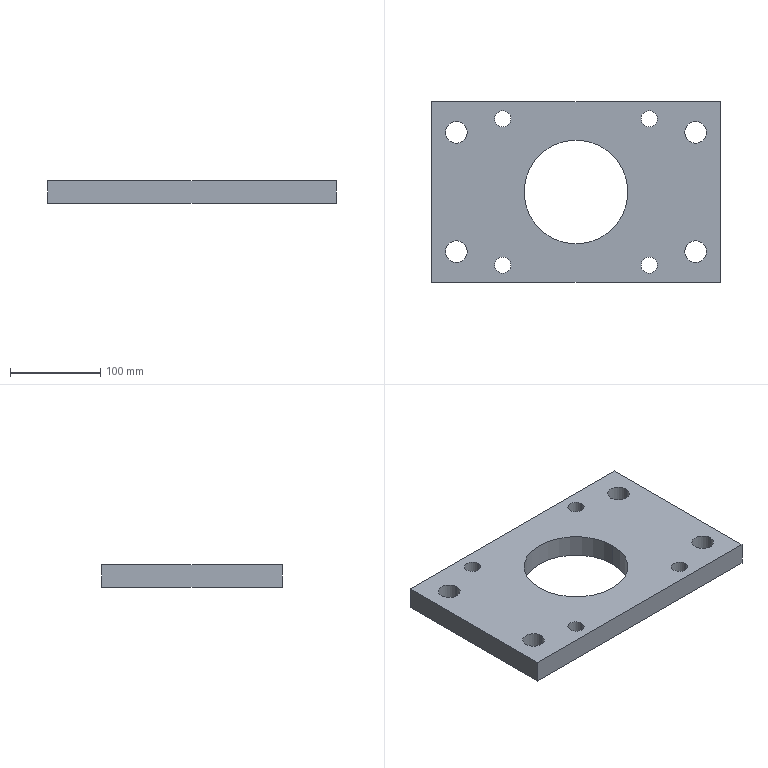Part | STEP file | CDS1FN180-250-A54Z_CS1-Flange | 1 solid | 24 faces | box 320 x 200 x 25 mm | volume 1269642 mm3 | cylinder 18 | plane 6 | commonest cylinder face diameters 18 x8 24 x8 115 x2